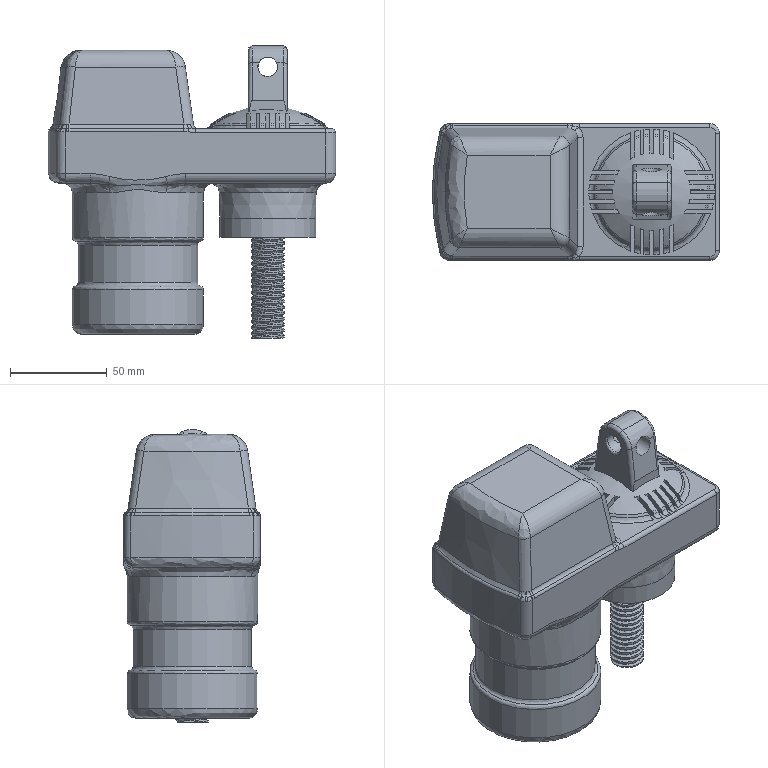Part | STEP file | J09 601A_default | 1 solid | 242 faces | box 148.1 x 70.5 x 151.812 mm | volume 777031 mm3 | spline 118 | plane 61 | cylinder 60 | cone 3 | commonest cylinder face diameters 40 x20 10 x11 4 x9 20 x5 10.1 x4 6 x3